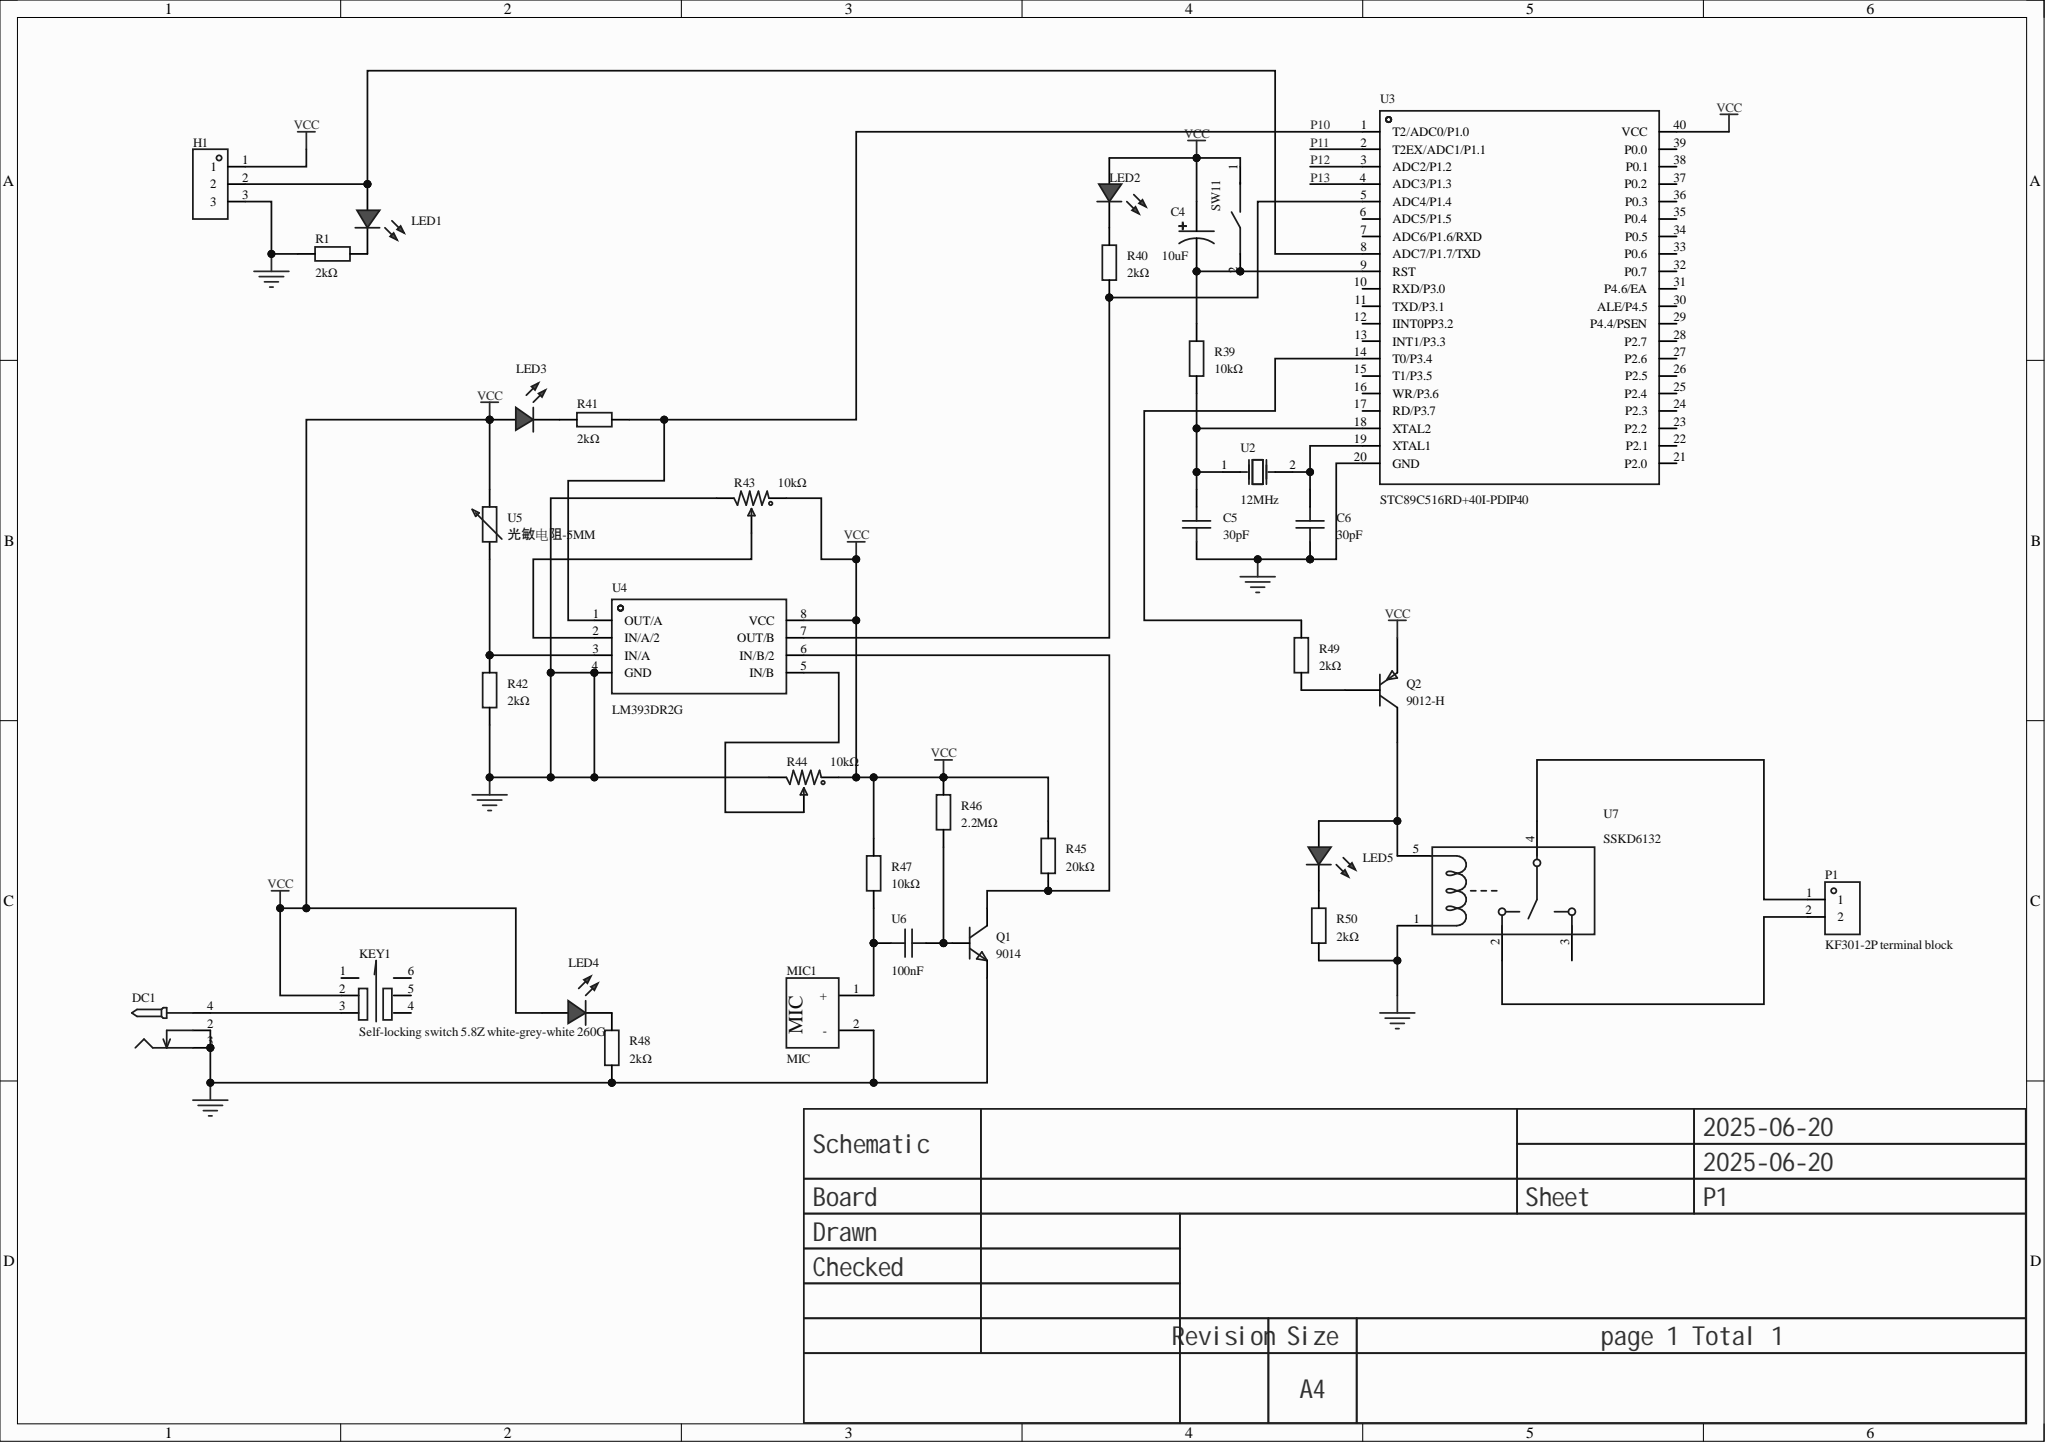Circuit board | Altium Designer | 35 parts | 25 nets
Bill of materials:
Comment,Description,Designator,Footprint,LibRef,Quantity
"10uF","Capacitance: 10uF; tolerance: ±20%; rated voltage: 250V; ripple current: -; equivalent series resistance: -;","C4","CAP-TH_BD6.3-P2.50-D1.0-FD","LKMC1202E100MF","1"
"30pF","Capacitance: 30pF; tolerance: ±5%; rated voltage: 50V; temperature coefficient: C0G;","C5, C6","CAP-TH_L3.6-W2.3-P5.00-D0.5","K300J10C0GF5UH5","2"
"","","DC1","DC-2.0","DC-005_2.0","1"
"","","H1","HDR-TH_3P-P2.54-V-M","HDR-M_2.54_1x3P","1"
"Self-locking switch 5.8Z white-grey-white 260G","Heat resistance 260 degrees","KEY1","SW-TH_6P-L5.8-W5.8-P2.00-LS4.5-TR","自锁开关 5.8Z白灰白260G","1"
"","","LED1, LED2, LED3, LED4, LED5","LED_TH-3mm","LED_TH-R_3mm","5"
"MIC","","MIC1","MIC-TH_BD6.0-P2.00","MIC","1"
"KF301-2P terminal block","","P1","CONN-TH_XY301V-A-5.0-2P","KF301-2P接线端子","1"
"9014","Transistor type: NPN; collector current (Ic): 100mA; collector-emitter breakdown voltage (Vceo): 45V; power dissipation (Pd): 450mW;","Q1","TO-92-3_L4.9-W3.7-P2.54-L","9014","1"
"9012-H","Transistor type: PNP; collector current (Ic): 500mA; collector-emitter breakdown voltage (Vceo): 20V; power dissipation (Pd): 625mW; DC current gain (hFE): 144@50mA,1V;","Q2","TO-92-3_L4.9-W3.7-P1.27-R","9012-H","1"
"2kΩ","","R1, R40, R41, R42, R48, R49, R50","Res_1/8W","Res_AXIAL-1/8W","7"
"10kΩ","","R39, R47","Res_1/8W","Res_AXIAL-1/8W","2"
"10kΩ","Resistance: 10kΩ; tolerance: ±25%; power: 100mW;","R43, R44","RES-ADJ-SMD_RM065-V1","RM065-103(10K)","2"
"20kΩ","","R45","Res_1/8W","Res_AXIAL-1/8W","1"
"2.2MΩ","","R46","Res_1/8W","Res_AXIAL-1/8W","1"
"Tact switch, 6*6*5 plastic head, 260G, travel 0.25mm, through-hole, middle 2 pins","","SW11","KEY-TH_2P-L6.0-W6.0-P5.00","轻触开关,6*6*5塑头,260G,行程0.25mm,直插中2脚","1"
"12MHz","Frequency: 12MHz; room-temperature frequency tolerance: ±30ppm; external load capacitance: -; frequency stability (full temperature): ±50ppm;","U2","HC-49US_L11.0-W4.6-P4.88","ECS-120-S-4","1"
"STC89C516RD+40I-PDIP40","CPU core: 51 series; program memory capacity: 61KB; total RAM: 1.25KB; GPIO port count: 35; operating voltage range: 3.5V~5.5V; max CPU frequency: -; program memory type: FLASH;","U3","DIP-40_L52.3-W13.9-P2.54-LS15.2-BL","STC89C516RD+40I-PDIP40","1"
"LM393DR2G","Comparators: dual; input offset voltage (Vos): 5mV; input bias current (Ib): 25nA;","U4","SOIC-8_L5.0-W4.0-P1.27-LS6.0-BL","LM393DR2G","1"
"光敏电阻-5MM","","U5","RES-TH_L4.9-W4.3-P3.4","光敏电阻-5MM","1"
"100nF","","U6","CAP-TH_L5.0-W2.5-P5.00-D1.0","100nF","1"
"SSKD6132","","U7","RELAY-TH_G2R-1","SSKD6132","1"
Netlist (Protel format):
[
C4
CAP-TH_BD6.3-P2.50-D1.0-FD
10uF



]
[
C5
CAP-TH_L3.6-W2.3-P5.00-D0.5
30pF



]
[
C6
CAP-TH_L3.6-W2.3-P5.00-D0.5
30pF



]
[
DC1
DC-2.0




]
[
H1
HDR-TH_3P-P2.54-V-M




]
[
KEY1
SW-TH_6P-L5.8-W5.8-P2.00-LS4.5-TR
Self-locking switch 5.8Z white-grey-white 260G



]
[
LED1
LED_TH-3mm




]
[
LED2
LED_TH-3mm




]
[
LED3
LED_TH-3mm




]
[
LED4
LED_TH-3mm




]
[
LED5
LED_TH-3mm




]
[
MIC1
MIC-TH_BD6.0-P2.00
MIC



]
[
P1
CONN-TH_XY301V-A-5.0-2P
KF301-2P terminal block



]
[
Q1
TO-92-3_L4.9-W3.7-P2.54-L
9014



]
[
Q2
TO-92-3_L4.9-W3.7-P1.27-R
9012-H



]
[
R1
Res_1/8W
2kΩ



]
[
R39
Res_1/8W
10kΩ



]
[
R40
Res_1/8W
2kΩ



]
[
R41
Res_1/8W
2kΩ



]
[
R42
Res_1/8W
2kΩ



]
[
R43
RES-ADJ-SMD_RM065-V1
10kΩ



]
[
R44
RES-ADJ-SMD_RM065-V1
10kΩ



]
[
R45
Res_1/8W
20kΩ



]
[
R46
Res_1/8W
2.2MΩ



]
[
R47
Res_1/8W
10kΩ



]
[
R48
Res_1/8W
2kΩ



]
[
R49
Res_1/8W
2kΩ



]
[
R50
Res_1/8W
2kΩ



]
[
SW11
KEY-TH_2P-L6.0-W6.0-P5.00
Tact switch, 6*6*5 plastic head, 260G, travel 0.25mm, through-hole, middle 2 pins



]
[
U2
HC-49US_L11.0-W4.6-P4.88
12MHz



]
[
U3
DIP-40_L52.3-W13.9-P2.54-LS15.2-BL
STC89C516RD+40I-PDIP40



]
[
U4
SOIC-8_L5.0-W4.0-P1.27-LS6.0-BL
LM393DR2G



]
[
U5
RES-TH_L4.9-W4.3-P3.4
光敏电阻-5MM



]
[
U6
CAP-TH_L5.0-W2.5-P5.00-D1.0
100nF



]
[
U7
RELAY-TH_G2R-1
SSKD6132



]
(
VCC
C4-1
H1-1
KEY1-2
LED2-1
LED3-1
LED4-1
Q2-3
R43-1
R44-1
R45-2
R46-2
R47-2
SW11-1
U3-40
U4-8
U5-2
)
(
P10
R41-2
U3-1
U4-1
)
(
NetR49_2
R49-2
U3-14
)
(
NetR44_2
R44-2
U4-5
)
(
NetR43_2
R43-2
U4-2
)
(
NetR42_2
R42-2
U4-3
U5-1
)
(
NetR40_1
R40-1
U3-5
U4-7
)
(
NetQ2_2
Q2-2
R49-1
)
(
NetQ1_3
Q1-3
R45-1
U4-6
)
(
NetQ1_2
Q1-2
R46-1
U6-1
)
(
NetP1_2
P1-2
U7-2
)
(
NetP1_1
P1-1
U7-4
)
(
NetMIC1_1
MIC1-1
R47-1
U6-2
)
(
NetLED5_2
LED5-2
R50-2
)
(
NetLED5_1
LED5-1
Q2-1
U7-5
)
(
NetLED4_2
LED4-2
R48-2
)
(
NetLED3_2
LED3-2
R41-1
)
(
NetLED2_2
LED2-2
R40-2
)
(
NetLED1_2
LED1-2
R1-2
)
(
NetH1_2
H1-2
LED1-1
U3-8
)
(
NetDC1_4
DC1-4
KEY1-3
)
(
NetC6_2
C6-2
U2-2
U3-19
)
(
NetC5_2
C5-2
R39-1
U2-1
U3-18
)
(
NetC4_2
C4-2
R39-2
SW11-2
U3-9
)
(
GND
C5-1
C6-1
DC1-2
DC1-3
H1-3
MIC1-2
Q1-1
R1-1
R42-1
R43-3
R44-3
R48-1
R50-1
U3-20
U4-4
U7-1
)